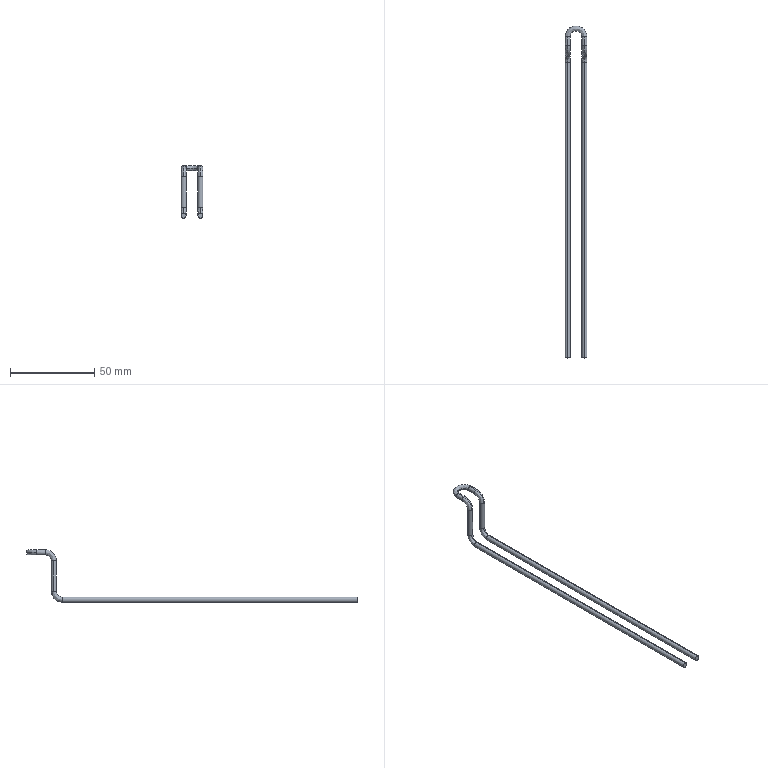Part | SolidWorks | features BaseBody 1 | 1 solid | 24 faces | box 13 x 196.5 x 31 mm | volume 3132 mm3 | cylinder 12 | spline 10 | plane 2 | commonest cylinder face diameters 3 x12
STEP:
#1=CARTESIAN_POINT('',(-10.,175.,-1.5));
#2=VERTEX_POINT('',#1);
#3=CARTESIAN_POINT('',(-10.,175.,1.5));
#4=VERTEX_POINT('',#3);
#5=CARTESIAN_POINT('',(-10.,175.,0.));
#6=DIRECTION('',(0.,-1.,0.));
#7=DIRECTION('',(0.,0.,-1.));
#8=AXIS2_PLACEMENT_3D('',#5,#6,#7);
#9=CIRCLE('',#8,1.5);
#10=EDGE_CURVE('',#2,#4,#9,.T.);
#11=ORIENTED_EDGE('',*,*,#10,.T.);
#12=CARTESIAN_POINT('',(-10.,0.,1.5));
#13=VERTEX_POINT('',#12);
#14=CARTESIAN_POINT('',(-10.,175.,1.5));
#15=DIRECTION('',(0.,-1.,0.));
#16=VECTOR('',#15,1000.);
#17=LINE('',#14,#16);
#18=EDGE_CURVE('',#4,#13,#17,.T.);
#19=ORIENTED_EDGE('',*,*,#18,.T.);
#20=CARTESIAN_POINT('',(-10.,0.,-1.5));
#21=VERTEX_POINT('',#20);
#22=CARTESIAN_POINT('',(-10.,0.,0.));
#23=DIRECTION('',(0.,1.,0.));
#24=DIRECTION('',(0.,0.,-1.));
#25=AXIS2_PLACEMENT_3D('',#22,#23,#24);
#26=CIRCLE('',#25,1.5);
#27=EDGE_CURVE('',#13,#21,#26,.T.);
#28=ORIENTED_EDGE('',*,*,#27,.T.);
#29=CARTESIAN_POINT('',(-10.,175.,-1.5));
#30=DIRECTION('',(0.,-1.,0.));
#31=VECTOR('',#30,1000.);
#32=LINE('',#29,#31);
#33=EDGE_CURVE('',#2,#21,#32,.T.);
#34=ORIENTED_EDGE('',*,*,#33,.F.);
#35=EDGE_LOOP('',(#11,#19,#28,#34));
#36=FACE_OUTER_BOUND('',#35,.T.);
#37=CARTESIAN_POINT('',(-10.,175.,0.));
#38=DIRECTION('',(0.,-1.,0.));
#39=DIRECTION('',(0.,0.,-1.));
#40=AXIS2_PLACEMENT_3D('',#37,#38,#39);
#41=CYLINDRICAL_SURFACE('',#40,1.5);
#42=ADVANCED_FACE('',(#36),#41,.T.);
#43=CARTESIAN_POINT('',(-10.,175.,0.));
#44=DIRECTION('',(0.,-1.,0.));
#45=DIRECTION('',(0.,0.,-1.));
#46=AXIS2_PLACEMENT_3D('',#43,#44,#45);
#47=CIRCLE('',#46,1.5);
#48=EDGE_CURVE('',#4,#2,#47,.T.);
#49=ORIENTED_EDGE('',*,*,#48,.F.);
#50=CARTESIAN_POINT('',(-10.,178.5,5.));
#51=VERTEX_POINT('',#50);
#52=CARTESIAN_POINT('',(-10.,175.,5.));
#53=DIRECTION('',(1.,0.,0.));
#54=DIRECTION('',(0.,0.,-1.));
#55=AXIS2_PLACEMENT_3D('',#52,#53,#54);
#56=CIRCLE('',#55,3.5);
#57=EDGE_CURVE('',#4,#51,#56,.T.);
#58=ORIENTED_EDGE('',*,*,#57,.T.);
#59=CARTESIAN_POINT('',(-11.5,180.,5.));
#60=VERTEX_POINT('',#59);
#61=CARTESIAN_POINT('',(-10.,180.,5.));
#62=DIRECTION('',(0.,0.,-1.));
#63=DIRECTION('',(0.,1.,0.));
#64=AXIS2_PLACEMENT_3D('',#61,#62,#63);
#65=CIRCLE('',#64,1.5);
#66=EDGE_CURVE('',#51,#60,#65,.T.);
#67=ORIENTED_EDGE('',*,*,#66,.T.);
#68=CARTESIAN_POINT('',(-10.,181.5,5.));
#69=VERTEX_POINT('',#68);
#70=CARTESIAN_POINT('',(-10.,180.,5.));
#71=DIRECTION('',(0.,0.,-1.));
#72=DIRECTION('',(0.,1.,0.));
#73=AXIS2_PLACEMENT_3D('',#70,#71,#72);
#74=CIRCLE('',#73,1.5);
#75=EDGE_CURVE('',#60,#69,#74,.T.);
#76=ORIENTED_EDGE('',*,*,#75,.T.);
#77=CARTESIAN_POINT('',(-10.,175.,5.));
#78=DIRECTION('',(1.,0.,0.));
#79=DIRECTION('',(0.,0.,-1.));
#80=AXIS2_PLACEMENT_3D('',#77,#78,#79);
#81=CIRCLE('',#80,6.5);
#82=EDGE_CURVE('',#2,#69,#81,.T.);
#83=ORIENTED_EDGE('',*,*,#82,.F.);
#84=EDGE_LOOP('',(#49,#58,#67,#76,#83));
#85=FACE_OUTER_BOUND('',#84,.T.);
#86=CARTESIAN_POINT('',(-10.,175.,-1.5));
#87=CARTESIAN_POINT('',(-10.,178.808,-1.5));
#88=CARTESIAN_POINT('',(-10.,181.5,1.192));
#89=CARTESIAN_POINT('',(-10.,181.5,5.));
#90=CARTESIAN_POINT('',(-13.,175.,-1.5));
#91=CARTESIAN_POINT('',(-13.,178.808,-1.5));
#92=CARTESIAN_POINT('',(-13.,181.5,1.192));
#93=CARTESIAN_POINT('',(-13.,181.5,5.));
#94=CARTESIAN_POINT('',(-13.,175.,1.5));
#95=CARTESIAN_POINT('',(-13.,177.05,1.5));
#96=CARTESIAN_POINT('',(-13.,178.5,2.95));
#97=CARTESIAN_POINT('',(-13.,178.5,5.));
#98=CARTESIAN_POINT('',(-10.,175.,1.5));
#99=CARTESIAN_POINT('',(-10.,177.05,1.5));
#100=CARTESIAN_POINT('',(-10.,178.5,2.95));
#101=CARTESIAN_POINT('',(-10.,178.5,5.));
#102=(BOUNDED_SURFACE()B_SPLINE_SURFACE(3,3,((#86,#87,#88,#89),(#90,#91,#92,#93),(#94,#95,#96,#97),(#98,#99,#100,#101)),.UNSPECIFIED.,.F.,.F.,.T.)B_SPLINE_SURFACE_WITH_KNOTS((4,4),(4,4),(0.,1.),(0.,1.),.UNSPECIFIED.)GEOMETRIC_REPRESENTATION_ITEM()RATIONAL_B_SPLINE_SURFACE(((1.,0.8047,0.8047,1.),(0.3333,0.2682,0.2682,0.3333),(0.3333,0.2682,0.2682,0.3333),(1.,0.8047,0.8047,1.)))REPRESENTATION_ITEM('')SURFACE());
#103=ADVANCED_FACE('',(#85),#102,.T.);
#104=ORIENTED_EDGE('',*,*,#75,.F.);
#105=CARTESIAN_POINT('',(-11.5,180.,23.));
#106=VERTEX_POINT('',#105);
#107=CARTESIAN_POINT('',(-11.5,180.,5.));
#108=DIRECTION('',(0.,0.,1.));
#109=VECTOR('',#108,1000.);
#110=LINE('',#107,#109);
#111=EDGE_CURVE('',#60,#106,#110,.T.);
#112=ORIENTED_EDGE('',*,*,#111,.T.);
#113=CARTESIAN_POINT('',(-10.,181.5,23.));
#114=VERTEX_POINT('',#113);
#115=CARTESIAN_POINT('',(-10.,180.,23.));
#116=DIRECTION('',(0.,0.,-1.));
#117=DIRECTION('',(1.,0.,0.));
#118=AXIS2_PLACEMENT_3D('',#115,#116,#117);
#119=CIRCLE('',#118,1.5);
#120=EDGE_CURVE('',#106,#114,#119,.T.);
#121=ORIENTED_EDGE('',*,*,#120,.T.);
#122=CARTESIAN_POINT('',(-8.5,180.,23.));
#123=VERTEX_POINT('',#122);
#124=CARTESIAN_POINT('',(-10.,180.,23.));
#125=DIRECTION('',(0.,0.,-1.));
#126=DIRECTION('',(1.,0.,0.));
#127=AXIS2_PLACEMENT_3D('',#124,#125,#126);
#128=CIRCLE('',#127,1.5);
#129=EDGE_CURVE('',#114,#123,#128,.T.);
#130=ORIENTED_EDGE('',*,*,#129,.T.);
#131=CARTESIAN_POINT('',(-8.5,180.,5.));
#132=VERTEX_POINT('',#131);
#133=CARTESIAN_POINT('',(-8.5,180.,5.));
#134=DIRECTION('',(0.,0.,1.));
#135=VECTOR('',#134,1000.);
#136=LINE('',#133,#135);
#137=EDGE_CURVE('',#132,#123,#136,.T.);
#138=ORIENTED_EDGE('',*,*,#137,.F.);
#139=CARTESIAN_POINT('',(-10.,180.,5.));
#140=DIRECTION('',(0.,0.,-1.));
#141=DIRECTION('',(0.,1.,0.));
#142=AXIS2_PLACEMENT_3D('',#139,#140,#141);
#143=CIRCLE('',#142,1.5);
#144=EDGE_CURVE('',#69,#132,#143,.T.);
#145=ORIENTED_EDGE('',*,*,#144,.F.);
#146=EDGE_LOOP('',(#104,#112,#121,#130,#138,#145));
#147=FACE_OUTER_BOUND('',#146,.T.);
#148=CARTESIAN_POINT('',(-10.,180.,5.));
#149=DIRECTION('',(0.,0.,1.));
#150=DIRECTION('',(1.,0.,0.));
#151=AXIS2_PLACEMENT_3D('',#148,#149,#150);
#152=CYLINDRICAL_SURFACE('',#151,1.5);
#153=ADVANCED_FACE('',(#147),#152,.T.);
#154=CARTESIAN_POINT('',(-10.,185.,29.5));
#155=VERTEX_POINT('',#154);
#156=CARTESIAN_POINT('',(-10.,185.,26.5));
#157=VERTEX_POINT('',#156);
#158=CARTESIAN_POINT('',(-10.,185.,28.));
#159=DIRECTION('',(0.,-1.,0.));
#160=DIRECTION('',(0.,0.,1.));
#161=AXIS2_PLACEMENT_3D('',#158,#159,#160);
#162=CIRCLE('',#161,1.5);
#163=EDGE_CURVE('',#155,#157,#162,.T.);
#164=ORIENTED_EDGE('',*,*,#163,.T.);
#165=CARTESIAN_POINT('',(-10.,185.,23.));
#166=DIRECTION('',(1.,0.,0.));
#167=DIRECTION('',(0.,-1.,0.));
#168=AXIS2_PLACEMENT_3D('',#165,#166,#167);
#169=CIRCLE('',#168,3.5);
#170=EDGE_CURVE('',#157,#114,#169,.T.);
#171=ORIENTED_EDGE('',*,*,#170,.T.);
#172=ORIENTED_EDGE('',*,*,#120,.F.);
#173=CARTESIAN_POINT('',(-10.,178.5,23.));
#174=VERTEX_POINT('',#173);
#175=CARTESIAN_POINT('',(-10.,180.,23.));
#176=DIRECTION('',(0.,0.,-1.));
#177=DIRECTION('',(1.,0.,0.));
#178=AXIS2_PLACEMENT_3D('',#175,#176,#177);
#179=CIRCLE('',#178,1.5);
#180=EDGE_CURVE('',#174,#106,#179,.T.);
#181=ORIENTED_EDGE('',*,*,#180,.F.);
#182=CARTESIAN_POINT('',(-10.,185.,23.));
#183=DIRECTION('',(1.,0.,0.));
#184=DIRECTION('',(0.,-1.,0.));
#185=AXIS2_PLACEMENT_3D('',#182,#183,#184);
#186=CIRCLE('',#185,6.5);
#187=EDGE_CURVE('',#155,#174,#186,.T.);
#188=ORIENTED_EDGE('',*,*,#187,.F.);
#189=EDGE_LOOP('',(#164,#171,#172,#181,#188));
#190=FACE_OUTER_BOUND('',#189,.T.);
#191=CARTESIAN_POINT('',(-10.,185.,29.5));
#192=CARTESIAN_POINT('',(-10.,181.192,29.5));
#193=CARTESIAN_POINT('',(-10.,178.5,26.808));
#194=CARTESIAN_POINT('',(-10.,178.5,23.));
#195=CARTESIAN_POINT('',(-13.,185.,29.5));
#196=CARTESIAN_POINT('',(-13.,181.192,29.5));
#197=CARTESIAN_POINT('',(-13.,178.5,26.808));
#198=CARTESIAN_POINT('',(-13.,178.5,23.));
#199=CARTESIAN_POINT('',(-13.,185.,26.5));
#200=CARTESIAN_POINT('',(-13.,182.95,26.5));
#201=CARTESIAN_POINT('',(-13.,181.5,25.05));
#202=CARTESIAN_POINT('',(-13.,181.5,23.));
#203=CARTESIAN_POINT('',(-10.,185.,26.5));
#204=CARTESIAN_POINT('',(-10.,182.95,26.5));
#205=CARTESIAN_POINT('',(-10.,181.5,25.05));
#206=CARTESIAN_POINT('',(-10.,181.5,23.));
#207=(BOUNDED_SURFACE()B_SPLINE_SURFACE(3,3,((#191,#192,#193,#194),(#195,#196,#197,#198),(#199,#200,#201,#202),(#203,#204,#205,#206)),.UNSPECIFIED.,.F.,.F.,.T.)B_SPLINE_SURFACE_WITH_KNOTS((4,4),(4,4),(0.,1.),(0.,1.),.UNSPECIFIED.)GEOMETRIC_REPRESENTATION_ITEM()RATIONAL_B_SPLINE_SURFACE(((1.,0.8047,0.8047,1.),(0.3333,0.2682,0.2682,0.3333),(0.3333,0.2682,0.2682,0.3333),(1.,0.8047,0.8047,1.)))REPRESENTATION_ITEM('')SURFACE());
#208=ADVANCED_FACE('',(#190),#207,.T.);
#209=CARTESIAN_POINT('',(-8.5,190.,28.));
#210=VERTEX_POINT('',#209);
#211=CARTESIAN_POINT('',(-10.,190.,29.5));
#212=VERTEX_POINT('',#211);
#213=CARTESIAN_POINT('',(-10.,190.,28.));
#214=DIRECTION('',(0.,-1.,0.));
#215=DIRECTION('',(0.,0.,-1.));
#216=AXIS2_PLACEMENT_3D('',#213,#214,#215);
#217=CIRCLE('',#216,1.5);
#218=EDGE_CURVE('',#210,#212,#217,.T.);
#219=ORIENTED_EDGE('',*,*,#218,.T.);
#220=CARTESIAN_POINT('',(-10.,190.,29.5));
#221=DIRECTION('',(0.,-1.,0.));
#222=VECTOR('',#221,1000.);
#223=LINE('',#220,#222);
#224=EDGE_CURVE('',#212,#155,#223,.T.);
#225=ORIENTED_EDGE('',*,*,#224,.T.);
#226=CARTESIAN_POINT('',(-8.5,185.,28.));
#227=VERTEX_POINT('',#226);
#228=CARTESIAN_POINT('',(-10.,185.,28.));
#229=DIRECTION('',(0.,-1.,0.));
#230=DIRECTION('',(0.,0.,1.));
#231=AXIS2_PLACEMENT_3D('',#228,#229,#230);
#232=CIRCLE('',#231,1.5);
#233=EDGE_CURVE('',#227,#155,#232,.T.);
#234=ORIENTED_EDGE('',*,*,#233,.F.);
#235=CARTESIAN_POINT('',(-10.,185.,28.));
#236=DIRECTION('',(0.,-1.,0.));
#237=DIRECTION('',(0.,0.,1.));
#238=AXIS2_PLACEMENT_3D('',#235,#236,#237);
#239=CIRCLE('',#238,1.5);
#240=EDGE_CURVE('',#157,#227,#239,.T.);
#241=ORIENTED_EDGE('',*,*,#240,.F.);
#242=CARTESIAN_POINT('',(-10.,190.,26.5));
#243=VERTEX_POINT('',#242);
#244=CARTESIAN_POINT('',(-10.,190.,26.5));
#245=DIRECTION('',(0.,-1.,0.));
#246=VECTOR('',#245,1000.);
#247=LINE('',#244,#246);
#248=EDGE_CURVE('',#243,#157,#247,.T.);
#249=ORIENTED_EDGE('',*,*,#248,.F.);
#250=CARTESIAN_POINT('',(-10.,190.,28.));
#251=DIRECTION('',(0.,-1.,0.));
#252=DIRECTION('',(0.,0.,-1.));
#253=AXIS2_PLACEMENT_3D('',#250,#251,#252);
#254=CIRCLE('',#253,1.5);
#255=EDGE_CURVE('',#243,#210,#254,.T.);
#256=ORIENTED_EDGE('',*,*,#255,.T.);
#257=EDGE_LOOP('',(#219,#225,#234,#241,#249,#256));
#258=FACE_OUTER_BOUND('',#257,.T.);
#259=CARTESIAN_POINT('',(-10.,190.,28.));
#260=DIRECTION('',(0.,-1.,0.));
#261=DIRECTION('',(0.,0.,-1.));
#262=AXIS2_PLACEMENT_3D('',#259,#260,#261);
#263=CYLINDRICAL_SURFACE('',#262,1.5);
#264=ADVANCED_FACE('',(#258),#263,.T.);
#265=CARTESIAN_POINT('',(0.,190.,26.5));
#266=VERTEX_POINT('',#265);
#267=CARTESIAN_POINT('',(-1.5,190.,28.));
#268=VERTEX_POINT('',#267);
#269=CARTESIAN_POINT('',(0.,190.,28.));
#270=DIRECTION('',(0.,1.,0.));
#271=DIRECTION('',(1.,0.,0.));
#272=AXIS2_PLACEMENT_3D('',#269,#270,#271);
#273=CIRCLE('',#272,1.5);
#274=EDGE_CURVE('',#266,#268,#273,.T.);
#275=ORIENTED_EDGE('',*,*,#274,.T.);
#276=CARTESIAN_POINT('',(-5.,190.,28.));
#277=DIRECTION('',(0.,0.,1.));
#278=DIRECTION('',(1.,0.,0.));
#279=AXIS2_PLACEMENT_3D('',#276,#277,#278);
#280=CIRCLE('',#279,3.5);
#281=EDGE_CURVE('',#268,#210,#280,.T.);
#282=ORIENTED_EDGE('',*,*,#281,.T.);
#283=ORIENTED_EDGE('',*,*,#255,.F.);
#284=CARTESIAN_POINT('',(-11.5,190.,28.));
#285=VERTEX_POINT('',#284);
#286=CARTESIAN_POINT('',(-10.,190.,28.));
#287=DIRECTION('',(0.,-1.,0.));
#288=DIRECTION('',(0.,0.,-1.));
#289=AXIS2_PLACEMENT_3D('',#286,#287,#288);
#290=CIRCLE('',#289,1.5);
#291=EDGE_CURVE('',#285,#243,#290,.T.);
#292=ORIENTED_EDGE('',*,*,#291,.F.);
#293=CARTESIAN_POINT('',(1.5,190.,28.));
#294=VERTEX_POINT('',#293);
#295=CARTESIAN_POINT('',(-5.,190.,28.));
#296=DIRECTION('',(0.,0.,1.));
#297=DIRECTION('',(1.,0.,0.));
#298=AXIS2_PLACEMENT_3D('',#295,#296,#297);
#299=CIRCLE('',#298,6.5);
#300=EDGE_CURVE('',#294,#285,#299,.T.);
#301=ORIENTED_EDGE('',*,*,#300,.F.);
#302=CARTESIAN_POINT('',(0.,190.,28.));
#303=DIRECTION('',(0.,1.,0.));
#304=DIRECTION('',(1.,0.,0.));
#305=AXIS2_PLACEMENT_3D('',#302,#303,#304);
#306=CIRCLE('',#305,1.5);
#307=EDGE_CURVE('',#294,#266,#306,.T.);
#308=ORIENTED_EDGE('',*,*,#307,.T.);
#309=EDGE_LOOP('',(#275,#282,#283,#292,#301,#308));
#310=FACE_OUTER_BOUND('',#309,.T.);
#311=CARTESIAN_POINT('',(1.5,190.,28.));
#312=CARTESIAN_POINT('',(1.5,203.,28.));
#313=CARTESIAN_POINT('',(-11.5,203.,28.));
#314=CARTESIAN_POINT('',(-11.5,190.,28.));
#315=CARTESIAN_POINT('',(1.5,190.,25.));
#316=CARTESIAN_POINT('',(1.5,203.,25.));
#317=CARTESIAN_POINT('',(-11.5,203.,25.));
#318=CARTESIAN_POINT('',(-11.5,190.,25.));
#319=CARTESIAN_POINT('',(-1.5,190.,25.));
#320=CARTESIAN_POINT('',(-1.5,197.,25.));
#321=CARTESIAN_POINT('',(-8.5,197.,25.));
#322=CARTESIAN_POINT('',(-8.5,190.,25.));
#323=CARTESIAN_POINT('',(-1.5,190.,28.));
#324=CARTESIAN_POINT('',(-1.5,197.,28.));
#325=CARTESIAN_POINT('',(-8.5,197.,28.));
#326=CARTESIAN_POINT('',(-8.5,190.,28.));
#327=(BOUNDED_SURFACE()B_SPLINE_SURFACE(3,3,((#311,#312,#313,#314),(#315,#316,#317,#318),(#319,#320,#321,#322),(#323,#324,#325,#326)),.UNSPECIFIED.,.F.,.F.,.T.)B_SPLINE_SURFACE_WITH_KNOTS((4,4),(4,4),(0.,1.),(0.,1.),.UNSPECIFIED.)GEOMETRIC_REPRESENTATION_ITEM()RATIONAL_B_SPLINE_SURFACE(((1.,0.3333,0.3333,1.),(0.3333,0.1111,0.1111,0.3333),(0.3333,0.1111,0.1111,0.3333),(1.,0.3333,0.3333,1.)))REPRESENTATION_ITEM('')SURFACE());
#328=ADVANCED_FACE('',(#310),#327,.T.);
#329=CARTESIAN_POINT('',(0.,185.,29.5));
#330=VERTEX_POINT('',#329);
#331=CARTESIAN_POINT('',(0.,185.,26.5));
#332=VERTEX_POINT('',#331);
#333=CARTESIAN_POINT('',(0.,185.,28.));
#334=DIRECTION('',(0.,1.,0.));
#335=DIRECTION('',(0.,0.,1.));
#336=AXIS2_PLACEMENT_3D('',#333,#334,#335);
#337=CIRCLE('',#336,1.5);
#338=EDGE_CURVE('',#330,#332,#337,.T.);
#339=ORIENTED_EDGE('',*,*,#338,.T.);
#340=CARTESIAN_POINT('',(0.,185.,26.5));
#341=DIRECTION('',(0.,1.,0.));
#342=VECTOR('',#341,1000.);
#343=LINE('',#340,#342);
#344=EDGE_CURVE('',#332,#266,#343,.T.);
#345=ORIENTED_EDGE('',*,*,#344,.T.);
#346=ORIENTED_EDGE('',*,*,#307,.F.);
#347=CARTESIAN_POINT('',(0.,190.,29.5));
#348=VERTEX_POINT('',#347);
#349=CARTESIAN_POINT('',(0.,190.,28.));
#350=DIRECTION('',(0.,1.,0.));
#351=DIRECTION('',(1.,0.,0.));
#352=AXIS2_PLACEMENT_3D('',#349,#350,#351);
#353=CIRCLE('',#352,1.5);
#354=EDGE_CURVE('',#348,#294,#353,.T.);
#355=ORIENTED_EDGE('',*,*,#354,.F.);
#356=CARTESIAN_POINT('',(0.,185.,29.5));
#357=DIRECTION('',(0.,1.,0.));
#358=VECTOR('',#357,1000.);
#359=LINE('',#356,#358);
#360=EDGE_CURVE('',#330,#348,#359,.T.);
#361=ORIENTED_EDGE('',*,*,#360,.F.);
#362=EDGE_LOOP('',(#339,#345,#346,#355,#361));
#363=FACE_OUTER_BOUND('',#362,.T.);
#364=CARTESIAN_POINT('',(0.,185.,28.));
#365=DIRECTION('',(0.,1.,0.));
#366=DIRECTION('',(0.,0.,1.));
#367=AXIS2_PLACEMENT_3D('',#364,#365,#366);
#368=CYLINDRICAL_SURFACE('',#367,1.5);
#369=ADVANCED_FACE('',(#363),#368,.T.);
#370=CARTESIAN_POINT('',(0.,185.,28.));
#371=DIRECTION('',(0.,1.,0.));
#372=DIRECTION('',(0.,0.,1.));
#373=AXIS2_PLACEMENT_3D('',#370,#371,#372);
#374=CIRCLE('',#373,1.5);
#375=EDGE_CURVE('',#332,#330,#374,.T.);
#376=ORIENTED_EDGE('',*,*,#375,.F.);
#377=CARTESIAN_POINT('',(0.,181.5,23.));
#378=VERTEX_POINT('',#377);
#379=CARTESIAN_POINT('',(0.,185.,23.));
#380=DIRECTION('',(1.,0.,0.));
#381=DIRECTION('',(0.,-1.,0.));
#382=AXIS2_PLACEMENT_3D('',#379,#380,#381);
#383=CIRCLE('',#382,3.5);
#384=EDGE_CURVE('',#332,#378,#383,.T.);
#385=ORIENTED_EDGE('',*,*,#384,.T.);
#386=CARTESIAN_POINT('',(-1.5,180.,23.));
#387=VERTEX_POINT('',#386);
#388=CARTESIAN_POINT('',(0.,180.,23.));
#389=DIRECTION('',(0.,0.,1.));
#390=DIRECTION('',(0.,-1.,0.));
#391=AXIS2_PLACEMENT_3D('',#388,#389,#390);
#392=CIRCLE('',#391,1.5);
#393=EDGE_CURVE('',#378,#387,#392,.T.);
#394=ORIENTED_EDGE('',*,*,#393,.T.);
#395=CARTESIAN_POINT('',(0.,178.5,23.));
#396=VERTEX_POINT('',#395);
#397=CARTESIAN_POINT('',(0.,180.,23.));
#398=DIRECTION('',(0.,0.,1.));
#399=DIRECTION('',(0.,-1.,0.));
#400=AXIS2_PLACEMENT_3D('',#397,#398,#399);
#401=CIRCLE('',#400,1.5);
#402=EDGE_CURVE('',#387,#396,#401,.T.);
#403=ORIENTED_EDGE('',*,*,#402,.T.);
#404=CARTESIAN_POINT('',(0.,185.,23.));
#405=DIRECTION('',(1.,0.,0.));
#406=DIRECTION('',(0.,-1.,0.));
#407=AXIS2_PLACEMENT_3D('',#404,#405,#406);
#408=CIRCLE('',#407,6.5);
#409=EDGE_CURVE('',#330,#396,#408,.T.);
#410=ORIENTED_EDGE('',*,*,#409,.F.);
#411=EDGE_LOOP('',(#376,#385,#394,#403,#410));
#412=FACE_OUTER_BOUND('',#411,.T.);
#413=CARTESIAN_POINT('',(0.,185.,29.5));
#414=CARTESIAN_POINT('',(0.,181.192,29.5));
#415=CARTESIAN_POINT('',(0.,178.5,26.808));
#416=CARTESIAN_POINT('',(0.,178.5,23.));
#417=CARTESIAN_POINT('',(-3.,185.,29.5));
#418=CARTESIAN_POINT('',(-3.,181.192,29.5));
#419=CARTESIAN_POINT('',(-3.,178.5,26.808));
#420=CARTESIAN_POINT('',(-3.,178.5,23.));
#421=CARTESIAN_POINT('',(-3.,185.,26.5));
#422=CARTESIAN_POINT('',(-3.,182.95,26.5));
#423=CARTESIAN_POINT('',(-3.,181.5,25.05));
#424=CARTESIAN_POINT('',(-3.,181.5,23.));
#425=CARTESIAN_POINT('',(0.,185.,26.5));
#426=CARTESIAN_POINT('',(0.,182.95,26.5));
#427=CARTESIAN_POINT('',(0.,181.5,25.05));
#428=CARTESIAN_POINT('',(0.,181.5,23.));
#429=(BOUNDED_SURFACE()B_SPLINE_SURFACE(3,3,((#413,#414,#415,#416),(#417,#418,#419,#420),(#421,#422,#423,#424),(#425,#426,#427,#428)),.UNSPECIFIED.,.F.,.F.,.T.)B_SPLINE_SURFACE_WITH_KNOTS((4,4),(4,4),(0.,1.),(0.,1.),.UNSPECIFIED.)GEOMETRIC_REPRESENTATION_ITEM()RATIONAL_B_SPLINE_SURFACE(((1.,0.8047,0.8047,1.),(0.3333,0.2682,0.2682,0.3333),(0.3333,0.2682,0.2682,0.3333),(1.,0.8047,0.8047,1.)))REPRESENTATION_ITEM('')SURFACE());
#430=ADVANCED_FACE('',(#412),#429,.T.);
#431=CARTESIAN_POINT('',(0.,181.5,5.));
#432=VERTEX_POINT('',#431);
#433=CARTESIAN_POINT('',(-1.5,180.,5.));
#434=VERTEX_POINT('',#433);
#435=CARTESIAN_POINT('',(0.,180.,5.));
#436=DIRECTION('',(0.,0.,1.));
#437=DIRECTION('',(1.,0.,0.));
#438=AXIS2_PLACEMENT_3D('',#435,#436,#437);
#439=CIRCLE('',#438,1.5);
#440=EDGE_CURVE('',#432,#434,#439,.T.);
#441=ORIENTED_EDGE('',*,*,#440,.T.);
#442=CARTESIAN_POINT('',(-1.5,180.,5.));
#443=DIRECTION('',(0.,0.,1.));
#444=VECTOR('',#443,1000.);
#445=LINE('',#442,#444);
#446=EDGE_CURVE('',#434,#387,#445,.T.);
#447=ORIENTED_EDGE('',*,*,#446,.T.);
#448=ORIENTED_EDGE('',*,*,#393,.F.);
#449=CARTESIAN_POINT('',(1.5,180.,23.));
#450=VERTEX_POINT('',#449);
#451=CARTESIAN_POINT('',(0.,180.,23.));
#452=DIRECTION('',(0.,0.,1.));
#453=DIRECTION('',(0.,-1.,0.));
#454=AXIS2_PLACEMENT_3D('',#451,#452,#453);
#455=CIRCLE('',#454,1.5);
#456=EDGE_CURVE('',#450,#378,#455,.T.);
#457=ORIENTED_EDGE('',*,*,#456,.F.);
#458=CARTESIAN_POINT('',(1.5,180.,5.));
#459=VERTEX_POINT('',#458);
#460=CARTESIAN_POINT('',(1.5,180.,5.));
#461=DIRECTION('',(0.,0.,1.));
#462=VECTOR('',#461,1000.);
#463=LINE('',#460,#462);
#464=EDGE_CURVE('',#459,#450,#463,.T.);
#465=ORIENTED_EDGE('',*,*,#464,.F.);
#466=CARTESIAN_POINT('',(0.,180.,5.));
#467=DIRECTION('',(0.,0.,1.));
#468=DIRECTION('',(1.,0.,0.));
#469=AXIS2_PLACEMENT_3D('',#466,#467,#468);
#470=CIRCLE('',#469,1.5);
#471=EDGE_CURVE('',#459,#432,#470,.T.);
#472=ORIENTED_EDGE('',*,*,#471,.T.);
#473=EDGE_LOOP('',(#441,#447,#448,#457,#465,#472));
#474=FACE_OUTER_BOUND('',#473,.T.);
#475=CARTESIAN_POINT('',(0.,180.,5.));
#476=DIRECTION('',(0.,0.,1.));
#477=DIRECTION('',(1.,0.,0.));
#478=AXIS2_PLACEMENT_3D('',#475,#476,#477);
#479=CYLINDRICAL_SURFACE('',#478,1.5);
#480=ADVANCED_FACE('',(#474),#479,.T.);
#481=CARTESIAN_POINT('',(0.,175.,-1.5));
#482=VERTEX_POINT('',#481);
#483=CARTESIAN_POINT('',(0.,175.,1.5));
#484=VERTEX_POINT('',#483);
#485=CARTESIAN_POINT('',(0.,175.,0.));
#486=DIRECTION('',(0.,1.,0.));
#487=DIRECTION('',(0.,0.,-1.));
#488=AXIS2_PLACEMENT_3D('',#485,#486,#487);
#489=CIRCLE('',#488,1.5);
#490=EDGE_CURVE('',#482,#484,#489,.T.);
#491=ORIENTED_EDGE('',*,*,#490,.T.);
#492=CARTESIAN_POINT('',(0.,178.5,5.));
#493=VERTEX_POINT('',#492);
#494=CARTESIAN_POINT('',(0.,175.,5.));
#495=DIRECTION('',(1.,0.,0.));
#496=DIRECTION('',(0.,0.,-1.));
#497=AXIS2_PLACEMENT_3D('',#494,#495,#496);
#498=CIRCLE('',#497,3.5);
#499=EDGE_CURVE('',#484,#493,#498,.T.);
#500=ORIENTED_EDGE('',*,*,#499,.T.);
#501=CARTESIAN_POINT('',(0.,180.,5.));
#502=DIRECTION('',(0.,0.,1.));
#503=DIRECTION('',(1.,0.,0.));
#504=AXIS2_PLACEMENT_3D('',#501,#502,#503);
#505=CIRCLE('',#504,1.5);
#506=EDGE_CURVE('',#434,#493,#505,.T.);
#507=ORIENTED_EDGE('',*,*,#506,.F.);
#508=ORIENTED_EDGE('',*,*,#440,.F.);
#509=CARTESIAN_POINT('',(0.,175.,5.));
#510=DIRECTION('',(1.,0.,0.));
#511=DIRECTION('',(0.,0.,-1.));
#512=AXIS2_PLACEMENT_3D('',#509,#510,#511);
#513=CIRCLE('',#512,6.5);
#514=EDGE_CURVE('',#482,#432,#513,.T.);
#515=ORIENTED_EDGE('',*,*,#514,.F.);
#516=EDGE_LOOP('',(#491,#500,#507,#508,#515));
#517=FACE_OUTER_BOUND('',#516,.T.);
#518=CARTESIAN_POINT('',(0.,175.,-1.5));
#519=CARTESIAN_POINT('',(0.,178.808,-1.5));
#520=CARTESIAN_POINT('',(0.,181.5,1.192));
#521=CARTESIAN_POINT('',(0.,181.5,5.));
#522=CARTESIAN_POINT('',(-3.,175.,-1.5));
#523=CARTESIAN_POINT('',(-3.,178.808,-1.5));
#524=CARTESIAN_POINT('',(-3.,181.5,1.192));
#525=CARTESIAN_POINT('',(-3.,181.5,5.));
#526=CARTESIAN_POINT('',(-3.,175.,1.5));
#527=CARTESIAN_POINT('',(-3.,177.05,1.5));
#528=CARTESIAN_POINT('',(-3.,178.5,2.95));
#529=CARTESIAN_POINT('',(-3.,178.5,5.));
#530=CARTESIAN_POINT('',(0.,175.,1.5));
#531=CARTESIAN_POINT('',(0.,177.05,1.5));
#532=CARTESIAN_POINT('',(0.,178.5,2.95));
#533=CARTESIAN_POINT('',(0.,178.5,5.));
#534=(BOUNDED_SURFACE()B_SPLINE_SURFACE(3,3,((#518,#519,#520,#521),(#522,#523,#524,#525),(#526,#527,#528,#529),(#530,#531,#532,#533)),.UNSPECIFIED.,.F.,.F.,.F.)B_SPLINE_SURFACE_WITH_KNOTS((4,4),(4,4),(0.,1.),(0.,1.),.UNSPECIFIED.)GEOMETRIC_REPRESENTATION_ITEM()RATIONAL_B_SPLINE_SURFACE(((1.,0.8047,0.8047,1.),(0.3333,0.2682,0.2682,0.3333),(0.3333,0.2682,0.2682,0.3333),(1.,0.8047,0.8047,1.)))REPRESENTATION_ITEM('')SURFACE());
#535=ADVANCED_FACE('',(#517),#534,.T.);
#536=CARTESIAN_POINT('',(0.,175.,0.));
#537=DIRECTION('',(0.,1.,0.));
#538=DIRECTION('',(0.,0.,-1.));
#539=AXIS2_PLACEMENT_3D('',#536,#537,#538);
#540=CIRCLE('',#539,1.5);
#541=EDGE_CURVE('',#484,#482,#540,.T.);
#542=ORIENTED_EDGE('',*,*,#541,.F.);
#543=CARTESIAN_POINT('',(0.,0.,1.5));
#544=VERTEX_POINT('',#543);
#545=CARTESIAN_POINT('',(0.,175.,1.5));
#546=DIRECTION('',(0.,-1.,0.));
#547=VECTOR('',#546,1000.);
#548=LINE('',#545,#547);
#549=EDGE_CURVE('',#484,#544,#548,.T.);
#550=ORIENTED_EDGE('',*,*,#549,.T.);
#551=CARTESIAN_POINT('',(0.,0.,-1.5));
#552=VERTEX_POINT('',#551);
#553=CARTESIAN_POINT('',(0.,0.,0.));
#554=DIRECTION('',(0.,1.,0.));
#555=DIRECTION('',(0.,0.,-1.));
#556=AXIS2_PLACEMENT_3D('',#553,#554,#555);
#557=CIRCLE('',#556,1.5);
#558=EDGE_CURVE('',#544,#552,#557,.T.);
#559=ORIENTED_EDGE('',*,*,#558,.T.);
#560=CARTESIAN_POINT('',(0.,175.,-1.5));
#561=DIRECTION('',(0.,-1.,0.));
#562=VECTOR('',#561,1000.);
#563=LINE('',#560,#562);
#564=EDGE_CURVE('',#482,#552,#563,.T.);
#565=ORIENTED_EDGE('',*,*,#564,.F.);
#566=EDGE_LOOP('',(#542,#550,#559,#565));
#567=FACE_OUTER_BOUND('',#566,.T.);
#568=CARTESIAN_POINT('',(0.,175.,0.));
#569=DIRECTION('',(0.,-1.,0.));
#570=DIRECTION('',(0.,0.,-1.));
#571=AXIS2_PLACEMENT_3D('',#568,#569,#570);
#572=CYLINDRICAL_SURFACE('',#571,1.5);
#573=ADVANCED_FACE('',(#567),#572,.T.);
#574=ORIENTED_EDGE('',*,*,#18,.F.);
#575=ORIENTED_EDGE('',*,*,#48,.T.);
#576=ORIENTED_EDGE('',*,*,#33,.T.);
#577=CARTESIAN_POINT('',(-10.,0.,0.));
#578=DIRECTION('',(0.,1.,0.));
#579=DIRECTION('',(0.,0.,-1.));
#580=AXIS2_PLACEMENT_3D('',#577,#578,#579);
#581=CIRCLE('',#580,1.5);
#582=EDGE_CURVE('',#21,#13,#581,.T.);
#583=ORIENTED_EDGE('',*,*,#582,.T.);
#584=EDGE_LOOP('',(#574,#575,#576,#583));
#585=FACE_OUTER_BOUND('',#584,.T.);
#586=CARTESIAN_POINT('',(-10.,175.,0.));
#587=DIRECTION('',(0.,-1.,0.));
#588=DIRECTION('',(0.,0.,-1.));
#589=AXIS2_PLACEMENT_3D('',#586,#587,#588);
#590=CYLINDRICAL_SURFACE('',#589,1.5);
#591=ADVANCED_FACE('',(#585),#590,.T.);
#592=ORIENTED_EDGE('',*,*,#57,.F.);
#593=ORIENTED_EDGE('',*,*,#10,.F.);
#594=ORIENTED_EDGE('',*,*,#82,.T.);
#595=ORIENTED_EDGE('',*,*,#144,.T.);
#596=CARTESIAN_POINT('',(-10.,180.,5.));
#597=DIRECTION('',(0.,0.,-1.));
#598=DIRECTION('',(0.,1.,0.));
#599=AXIS2_PLACEMENT_3D('',#596,#597,#598);
#600=CIRCLE('',#599,1.5);
#601=EDGE_CURVE('',#132,#51,#600,.T.);
#602=ORIENTED_EDGE('',*,*,#601,.T.);
#603=EDGE_LOOP('',(#592,#593,#594,#595,#602));
#604=FACE_OUTER_BOUND('',#603,.T.);
#605=CARTESIAN_POINT('',(-10.,175.,1.5));
#606=CARTESIAN_POINT('',(-10.,177.05,1.5));
#607=CARTESIAN_POINT('',(-10.,178.5,2.95));
#608=CARTESIAN_POINT('',(-10.,178.5,5.));
#609=CARTESIAN_POINT('',(-7.,175.,1.5));
#610=CARTESIAN_POINT('',(-7.,177.05,1.5));
#611=CARTESIAN_POINT('',(-7.,178.5,2.95));
#612=CARTESIAN_POINT('',(-7.,178.5,5.));
#613=CARTESIAN_POINT('',(-7.,175.,-1.5));
#614=CARTESIAN_POINT('',(-7.,178.808,-1.5));
#615=CARTESIAN_POINT('',(-7.,181.5,1.192));
#616=CARTESIAN_POINT('',(-7.,181.5,5.));
#617=CARTESIAN_POINT('',(-10.,175.,-1.5));
#618=CARTESIAN_POINT('',(-10.,178.808,-1.5));
#619=CARTESIAN_POINT('',(-10.,181.5,1.192));
#620=CARTESIAN_POINT('',(-10.,181.5,5.));
#621=(BOUNDED_SURFACE()B_SPLINE_SURFACE(3,3,((#605,#606,#607,#608),(#609,#610,#611,#612),(#613,#614,#615,#616),(#617,#618,#619,#620)),.UNSPECIFIED.,.F.,.F.,.F.)B_SPLINE_SURFACE_WITH_KNOTS((4,4),(4,4),(0.,1.),(0.,1.),.UNSPECIFIED.)GEOMETRIC_REPRESENTATION_ITEM()RATIONAL_B_SPLINE_SURFACE(((1.,0.8047,0.8047,1.),(0.3333,0.2682,0.2682,0.3333),(0.3333,0.2682,0.2682,0.3333),(1.,0.8047,0.8047,1.)))REPRESENTATION_ITEM('')SURFACE());
#622=ADVANCED_FACE('',(#604),#621,.T.);
#623=ORIENTED_EDGE('',*,*,#582,.F.);
#624=ORIENTED_EDGE('',*,*,#27,.F.);
#625=EDGE_LOOP('',(#623,#624));
#626=FACE_OUTER_BOUND('',#625,.T.);
#627=CARTESIAN_POINT('',(-10.,0.,0.));
#628=DIRECTION('',(0.,1.,0.));
#629=DIRECTION('',(0.,0.,1.));
#630=AXIS2_PLACEMENT_3D('',#627,#628,#629);
#631=PLANE('',#630);
#632=ADVANCED_FACE('',(#626),#631,.F.);
#633=ORIENTED_EDGE('',*,*,#111,.F.);
#634=ORIENTED_EDGE('',*,*,#66,.F.);
#635=ORIENTED_EDGE('',*,*,#601,.F.);
#636=ORIENTED_EDGE('',*,*,#137,.T.);
#637=CARTESIAN_POINT('',(-10.,180.,23.));
#638=DIRECTION('',(0.,0.,-1.));
#639=DIRECTION('',(1.,0.,0.));
#640=AXIS2_PLACEMENT_3D('',#637,#638,#639);
#641=CIRCLE('',#640,1.5);
#642=EDGE_CURVE('',#123,#174,#641,.T.);
#643=ORIENTED_EDGE('',*,*,#642,.T.);
#644=ORIENTED_EDGE('',*,*,#180,.T.);
#645=EDGE_LOOP('',(#633,#634,#635,#636,#643,#644));
#646=FACE_OUTER_BOUND('',#645,.T.);
#647=CARTESIAN_POINT('',(-10.,180.,5.));
#648=DIRECTION('',(0.,0.,1.));
#649=DIRECTION('',(1.,0.,0.));
#650=AXIS2_PLACEMENT_3D('',#647,#648,#649);
#651=CYLINDRICAL_SURFACE('',#650,1.5);
#652=ADVANCED_FACE('',(#646),#651,.T.);
#653=ORIENTED_EDGE('',*,*,#170,.F.);
#654=ORIENTED_EDGE('',*,*,#240,.T.);
#655=ORIENTED_EDGE('',*,*,#233,.T.);
#656=ORIENTED_EDGE('',*,*,#187,.T.);
#657=ORIENTED_EDGE('',*,*,#642,.F.);
#658=ORIENTED_EDGE('',*,*,#129,.F.);
#659=EDGE_LOOP('',(#653,#654,#655,#656,#657,#658));
#660=FACE_OUTER_BOUND('',#659,.T.);
#661=CARTESIAN_POINT('',(-10.,185.,26.5));
#662=CARTESIAN_POINT('',(-10.,182.95,26.5));
#663=CARTESIAN_POINT('',(-10.,181.5,25.05));
#664=CARTESIAN_POINT('',(-10.,181.5,23.));
#665=CARTESIAN_POINT('',(-9.121,185.,26.5));
#666=CARTESIAN_POINT('',(-9.121,182.95,26.5));
#667=CARTESIAN_POINT('',(-9.121,181.5,25.05));
#668=CARTESIAN_POINT('',(-9.121,181.5,23.));
#669=CARTESIAN_POINT('',(-8.5,185.,27.121));
#670=CARTESIAN_POINT('',(-8.5,182.586,27.121));
#671=CARTESIAN_POINT('',(-8.5,180.879,25.414));
#672=CARTESIAN_POINT('',(-8.5,180.879,23.));
#673=CARTESIAN_POINT('',(-8.5,185.,28.));
#674=CARTESIAN_POINT('',(-8.5,182.071,28.));
#675=CARTESIAN_POINT('',(-8.5,180.,25.929));
#676=CARTESIAN_POINT('',(-8.5,180.,23.));
#677=CARTESIAN_POINT('',(-8.5,185.,28.879));
#678=CARTESIAN_POINT('',(-8.5,181.556,28.879));
#679=CARTESIAN_POINT('',(-8.5,179.121,26.444));
#680=CARTESIAN_POINT('',(-8.5,179.121,23.));
#681=CARTESIAN_POINT('',(-9.121,185.,29.5));
#682=CARTESIAN_POINT('',(-9.121,181.192,29.5));
#683=CARTESIAN_POINT('',(-9.121,178.5,26.808));
#684=CARTESIAN_POINT('',(-9.121,178.5,23.));
#685=CARTESIAN_POINT('',(-10.,185.,29.5));
#686=CARTESIAN_POINT('',(-10.,181.192,29.5));
#687=CARTESIAN_POINT('',(-10.,178.5,26.808));
#688=CARTESIAN_POINT('',(-10.,178.5,23.));
#689=(BOUNDED_SURFACE()B_SPLINE_SURFACE(3,3,((#661,#662,#663,#664),(#665,#666,#667,#668),(#669,#670,#671,#672),(#673,#674,#675,#676),(#677,#678,#679,#680),(#681,#682,#683,#684),(#685,#686,#687,#688)),.UNSPECIFIED.,.F.,.F.,.T.)B_SPLINE_SURFACE_WITH_KNOTS((4,3,4),(4,4),(0.,0.5,1.),(0.,1.),.UNSPECIFIED.)GEOMETRIC_REPRESENTATION_ITEM()RATIONAL_B_SPLINE_SURFACE(((1.,0.8047,0.8047,1.),(0.8047,0.6476,0.6476,0.8047),(0.8047,0.6476,0.6476,0.8047),(1.,0.8047,0.8047,1.),(0.8047,0.6476,0.6476,0.8047),(0.8047,0.6476,0.6476,0.8047),(1.,0.8047,0.8047,1.)))REPRESENTATION_ITEM('')SURFACE());
#690=ADVANCED_FACE('',(#660),#689,.T.);
#691=ORIENTED_EDGE('',*,*,#224,.F.);
#692=CARTESIAN_POINT('',(-10.,190.,28.));
#693=DIRECTION('',(0.,-1.,0.));
#694=DIRECTION('',(0.,0.,-1.));
#695=AXIS2_PLACEMENT_3D('',#692,#693,#694);
#696=CIRCLE('',#695,1.5);
#697=EDGE_CURVE('',#212,#285,#696,.T.);
#698=ORIENTED_EDGE('',*,*,#697,.T.);
#699=ORIENTED_EDGE('',*,*,#291,.T.);
#700=ORIENTED_EDGE('',*,*,#248,.T.);
#701=ORIENTED_EDGE('',*,*,#163,.F.);
#702=EDGE_LOOP('',(#691,#698,#699,#700,#701));
#703=FACE_OUTER_BOUND('',#702,.T.);
#704=CARTESIAN_POINT('',(-10.,190.,28.));
#705=DIRECTION('',(0.,-1.,0.));
#706=DIRECTION('',(0.,0.,-1.));
#707=AXIS2_PLACEMENT_3D('',#704,#705,#706);
#708=CYLINDRICAL_SURFACE('',#707,1.5);
#709=ADVANCED_FACE('',(#703),#708,.T.);
#710=ORIENTED_EDGE('',*,*,#281,.F.);
#711=CARTESIAN_POINT('',(0.,190.,28.));
#712=DIRECTION('',(0.,1.,0.));
#713=DIRECTION('',(1.,0.,0.));
#714=AXIS2_PLACEMENT_3D('',#711,#712,#713);
#715=CIRCLE('',#714,1.5);
#716=EDGE_CURVE('',#268,#348,#715,.T.);
#717=ORIENTED_EDGE('',*,*,#716,.T.);
#718=ORIENTED_EDGE('',*,*,#354,.T.);
#719=ORIENTED_EDGE('',*,*,#300,.T.);
#720=ORIENTED_EDGE('',*,*,#697,.F.);
#721=ORIENTED_EDGE('',*,*,#218,.F.);
#722=EDGE_LOOP('',(#710,#717,#718,#719,#720,#721));
#723=FACE_OUTER_BOUND('',#722,.T.);
#724=CARTESIAN_POINT('',(-1.5,190.,28.));
#725=CARTESIAN_POINT('',(-1.5,197.,28.));
#726=CARTESIAN_POINT('',(-8.5,197.,28.));
#727=CARTESIAN_POINT('',(-8.5,190.,28.));
#728=CARTESIAN_POINT('',(-1.5,190.,31.));
#729=CARTESIAN_POINT('',(-1.5,197.,31.));
#730=CARTESIAN_POINT('',(-8.5,197.,31.));
#731=CARTESIAN_POINT('',(-8.5,190.,31.));
#732=CARTESIAN_POINT('',(1.5,190.,31.));
#733=CARTESIAN_POINT('',(1.5,203.,31.));
#734=CARTESIAN_POINT('',(-11.5,203.,31.));
#735=CARTESIAN_POINT('',(-11.5,190.,31.));
#736=CARTESIAN_POINT('',(1.5,190.,28.));
#737=CARTESIAN_POINT('',(1.5,203.,28.));
#738=CARTESIAN_POINT('',(-11.5,203.,28.));
#739=CARTESIAN_POINT('',(-11.5,190.,28.));
#740=(BOUNDED_SURFACE()B_SPLINE_SURFACE(3,3,((#724,#725,#726,#727),(#728,#729,#730,#731),(#732,#733,#734,#735),(#736,#737,#738,#739)),.UNSPECIFIED.,.F.,.F.,.T.)B_SPLINE_SURFACE_WITH_KNOTS((4,4),(4,4),(0.,1.),(0.,1.),.UNSPECIFIED.)GEOMETRIC_REPRESENTATION_ITEM()RATIONAL_B_SPLINE_SURFACE(((1.,0.3333,0.3333,1.),(0.3333,0.1111,0.1111,0.3333),(0.3333,0.1111,0.1111,0.3333),(1.,0.3333,0.3333,1.)))REPRESENTATION_ITEM('')SURFACE());
#741=ADVANCED_FACE('',(#723),#740,.T.);
#742=ORIENTED_EDGE('',*,*,#344,.F.);
#743=ORIENTED_EDGE('',*,*,#375,.T.);
#744=ORIENTED_EDGE('',*,*,#360,.T.);
#745=ORIENTED_EDGE('',*,*,#716,.F.);
#746=ORIENTED_EDGE('',*,*,#274,.F.);
#747=EDGE_LOOP('',(#742,#743,#744,#745,#746));
#748=FACE_OUTER_BOUND('',#747,.T.);
#749=CARTESIAN_POINT('',(0.,185.,28.));
#750=DIRECTION('',(0.,1.,0.));
#751=DIRECTION('',(0.,0.,1.));
#752=AXIS2_PLACEMENT_3D('',#749,#750,#751);
#753=CYLINDRICAL_SURFACE('',#752,1.5);
#754=ADVANCED_FACE('',(#748),#753,.T.);
#755=ORIENTED_EDGE('',*,*,#384,.F.);
#756=ORIENTED_EDGE('',*,*,#338,.F.);
#757=ORIENTED_EDGE('',*,*,#409,.T.);
#758=CARTESIAN_POINT('',(0.,180.,23.));
#759=DIRECTION('',(0.,0.,1.));
#760=DIRECTION('',(0.,-1.,0.));
#761=AXIS2_PLACEMENT_3D('',#758,#759,#760);
#762=CIRCLE('',#761,1.5);
#763=EDGE_CURVE('',#396,#450,#762,.T.);
#764=ORIENTED_EDGE('',*,*,#763,.T.);
#765=ORIENTED_EDGE('',*,*,#456,.T.);
#766=EDGE_LOOP('',(#755,#756,#757,#764,#765));
#767=FACE_OUTER_BOUND('',#766,.T.);
#768=CARTESIAN_POINT('',(0.,185.,26.5));
#769=CARTESIAN_POINT('',(0.,182.95,26.5));
#770=CARTESIAN_POINT('',(0.,181.5,25.05));
#771=CARTESIAN_POINT('',(0.,181.5,23.));
#772=CARTESIAN_POINT('',(3.,185.,26.5));
#773=CARTESIAN_POINT('',(3.,182.95,26.5));
#774=CARTESIAN_POINT('',(3.,181.5,25.05));
#775=CARTESIAN_POINT('',(3.,181.5,23.));
#776=CARTESIAN_POINT('',(3.,185.,29.5));
#777=CARTESIAN_POINT('',(3.,181.192,29.5));
#778=CARTESIAN_POINT('',(3.,178.5,26.808));
#779=CARTESIAN_POINT('',(3.,178.5,23.));
#780=CARTESIAN_POINT('',(0.,185.,29.5));
#781=CARTESIAN_POINT('',(0.,181.192,29.5));
#782=CARTESIAN_POINT('',(0.,178.5,26.808));
#783=CARTESIAN_POINT('',(0.,178.5,23.));
#784=(BOUNDED_SURFACE()B_SPLINE_SURFACE(3,3,((#768,#769,#770,#771),(#772,#773,#774,#775),(#776,#777,#778,#779),(#780,#781,#782,#783)),.UNSPECIFIED.,.F.,.F.,.T.)B_SPLINE_SURFACE_WITH_KNOTS((4,4),(4,4),(0.,1.),(0.,1.),.UNSPECIFIED.)GEOMETRIC_REPRESENTATION_ITEM()RATIONAL_B_SPLINE_SURFACE(((1.,0.8047,0.8047,1.),(0.3333,0.2682,0.2682,0.3333),(0.3333,0.2682,0.2682,0.3333),(1.,0.8047,0.8047,1.)))REPRESENTATION_ITEM('')SURFACE());
#785=ADVANCED_FACE('',(#767),#784,.T.);
#786=ORIENTED_EDGE('',*,*,#446,.F.);
#787=ORIENTED_EDGE('',*,*,#506,.T.);
#788=CARTESIAN_POINT('',(0.,180.,5.));
#789=DIRECTION('',(0.,0.,1.));
#790=DIRECTION('',(1.,0.,0.));
#791=AXIS2_PLACEMENT_3D('',#788,#789,#790);
#792=CIRCLE('',#791,1.5);
#793=EDGE_CURVE('',#493,#459,#792,.T.);
#794=ORIENTED_EDGE('',*,*,#793,.T.);
#795=ORIENTED_EDGE('',*,*,#464,.T.);
#796=ORIENTED_EDGE('',*,*,#763,.F.);
#797=ORIENTED_EDGE('',*,*,#402,.F.);
#798=EDGE_LOOP('',(#786,#787,#794,#795,#796,#797));
#799=FACE_OUTER_BOUND('',#798,.T.);
#800=CARTESIAN_POINT('',(0.,180.,5.));
#801=DIRECTION('',(0.,0.,1.));
#802=DIRECTION('',(1.,0.,0.));
#803=AXIS2_PLACEMENT_3D('',#800,#801,#802);
#804=CYLINDRICAL_SURFACE('',#803,1.5);
#805=ADVANCED_FACE('',(#799),#804,.T.);
#806=ORIENTED_EDGE('',*,*,#499,.F.);
#807=ORIENTED_EDGE('',*,*,#541,.T.);
#808=ORIENTED_EDGE('',*,*,#514,.T.);
#809=ORIENTED_EDGE('',*,*,#471,.F.);
#810=ORIENTED_EDGE('',*,*,#793,.F.);
#811=EDGE_LOOP('',(#806,#807,#808,#809,#810));
#812=FACE_OUTER_BOUND('',#811,.T.);
#813=CARTESIAN_POINT('',(0.,175.,1.5));
#814=CARTESIAN_POINT('',(0.,177.05,1.5));
#815=CARTESIAN_POINT('',(0.,178.5,2.95));
#816=CARTESIAN_POINT('',(0.,178.5,5.));
#817=CARTESIAN_POINT('',(0.8787,175.,1.5));
#818=CARTESIAN_POINT('',(0.8787,177.05,1.5));
#819=CARTESIAN_POINT('',(0.8787,178.5,2.95));
#820=CARTESIAN_POINT('',(0.8787,178.5,5.));
#821=CARTESIAN_POINT('',(1.5,175.,0.8787));
#822=CARTESIAN_POINT('',(1.5,177.414,0.8787));
#823=CARTESIAN_POINT('',(1.5,179.121,2.586));
#824=CARTESIAN_POINT('',(1.5,179.121,5.));
#825=CARTESIAN_POINT('',(1.5,175.,0.));
#826=CARTESIAN_POINT('',(1.5,177.929,0.));
#827=CARTESIAN_POINT('',(1.5,180.,2.071));
#828=CARTESIAN_POINT('',(1.5,180.,5.));
#829=CARTESIAN_POINT('',(1.5,175.,-0.8787));
#830=CARTESIAN_POINT('',(1.5,178.444,-0.8787));
#831=CARTESIAN_POINT('',(1.5,180.879,1.556));
#832=CARTESIAN_POINT('',(1.5,180.879,5.));
#833=CARTESIAN_POINT('',(0.8787,175.,-1.5));
#834=CARTESIAN_POINT('',(0.8787,178.808,-1.5));
#835=CARTESIAN_POINT('',(0.8787,181.5,1.192));
#836=CARTESIAN_POINT('',(0.8787,181.5,5.));
#837=CARTESIAN_POINT('',(0.,175.,-1.5));
#838=CARTESIAN_POINT('',(0.,178.808,-1.5));
#839=CARTESIAN_POINT('',(0.,181.5,1.192));
#840=CARTESIAN_POINT('',(0.,181.5,5.));
#841=(BOUNDED_SURFACE()B_SPLINE_SURFACE(3,3,((#813,#814,#815,#816),(#817,#818,#819,#820),(#821,#822,#823,#824),(#825,#826,#827,#828),(#829,#830,#831,#832),(#833,#834,#835,#836),(#837,#838,#839,#840)),.UNSPECIFIED.,.F.,.F.,.F.)B_SPLINE_SURFACE_WITH_KNOTS((4,3,4),(4,4),(0.,0.5,1.),(0.,1.),.UNSPECIFIED.)GEOMETRIC_REPRESENTATION_ITEM()RATIONAL_B_SPLINE_SURFACE(((1.,0.8047,0.8047,1.),(0.8047,0.6476,0.6476,0.8047),(0.8047,0.6476,0.6476,0.8047),(1.,0.8047,0.8047,1.),(0.8047,0.6476,0.6476,0.8047),(0.8047,0.6476,0.6476,0.8047),(1.,0.8047,0.8047,1.)))REPRESENTATION_ITEM('')SURFACE());
#842=ADVANCED_FACE('',(#812),#841,.T.);
#843=ORIENTED_EDGE('',*,*,#549,.F.);
#844=ORIENTED_EDGE('',*,*,#490,.F.);
#845=ORIENTED_EDGE('',*,*,#564,.T.);
#846=CARTESIAN_POINT('',(0.,0.,0.));
#847=DIRECTION('',(0.,1.,0.));
#848=DIRECTION('',(0.,0.,-1.));
#849=AXIS2_PLACEMENT_3D('',#846,#847,#848);
#850=CIRCLE('',#849,1.5);
#851=EDGE_CURVE('',#552,#544,#850,.T.);
#852=ORIENTED_EDGE('',*,*,#851,.T.);
#853=EDGE_LOOP('',(#843,#844,#845,#852));
#854=FACE_OUTER_BOUND('',#853,.T.);
#855=CARTESIAN_POINT('',(0.,175.,0.));
#856=DIRECTION('',(0.,-1.,0.));
#857=DIRECTION('',(0.,0.,-1.));
#858=AXIS2_PLACEMENT_3D('',#855,#856,#857);
#859=CYLINDRICAL_SURFACE('',#858,1.5);
#860=ADVANCED_FACE('',(#854),#859,.T.);
#861=ORIENTED_EDGE('',*,*,#851,.F.);
#862=ORIENTED_EDGE('',*,*,#558,.F.);
#863=EDGE_LOOP('',(#861,#862));
#864=FACE_OUTER_BOUND('',#863,.T.);
#865=CARTESIAN_POINT('',(0.,0.,0.));
#866=DIRECTION('',(0.,1.,0.));
#867=DIRECTION('',(0.,0.,1.));
#868=AXIS2_PLACEMENT_3D('',#865,#866,#867);
#869=PLANE('',#868);
#870=ADVANCED_FACE('',(#864),#869,.F.);
#871=CLOSED_SHELL('',(#42,#103,#153,#208,#264,#328,#369,#430,#480,#535,#573,#591,#622,#632,#652,#690,#709,#741,#754,#785,#805,#842,#860,#870));
#872=MANIFOLD_SOLID_BREP('',#871);
#873=CARTESIAN_POINT('',(0.,0.,0.));
#874=DIRECTION('',(0.,0.,1.));
#875=DIRECTION('',(1.,0.,0.));
#876=AXIS2_PLACEMENT_3D('',#873,#874,#875);
#877=(LENGTH_UNIT()NAMED_UNIT(*)SI_UNIT(.MILLI.,.METRE.));
#878=UNCERTAINTY_MEASURE_WITH_UNIT(LENGTH_MEASURE(0.00001),#877,'','');
#879=(NAMED_UNIT(*)PLANE_ANGLE_UNIT()SI_UNIT($,.RADIAN.));
#880=(NAMED_UNIT(*)SI_UNIT($,.STERADIAN.)SOLID_ANGLE_UNIT());
#881=(GEOMETRIC_REPRESENTATION_CONTEXT(3)GLOBAL_UNCERTAINTY_ASSIGNED_CONTEXT((#878))GLOBAL_UNIT_ASSIGNED_CONTEXT((#877,#879,#880))REPRESENTATION_CONTEXT('',''));
#882=ADVANCED_BREP_SHAPE_REPRESENTATION('',(#872,#876),#881);